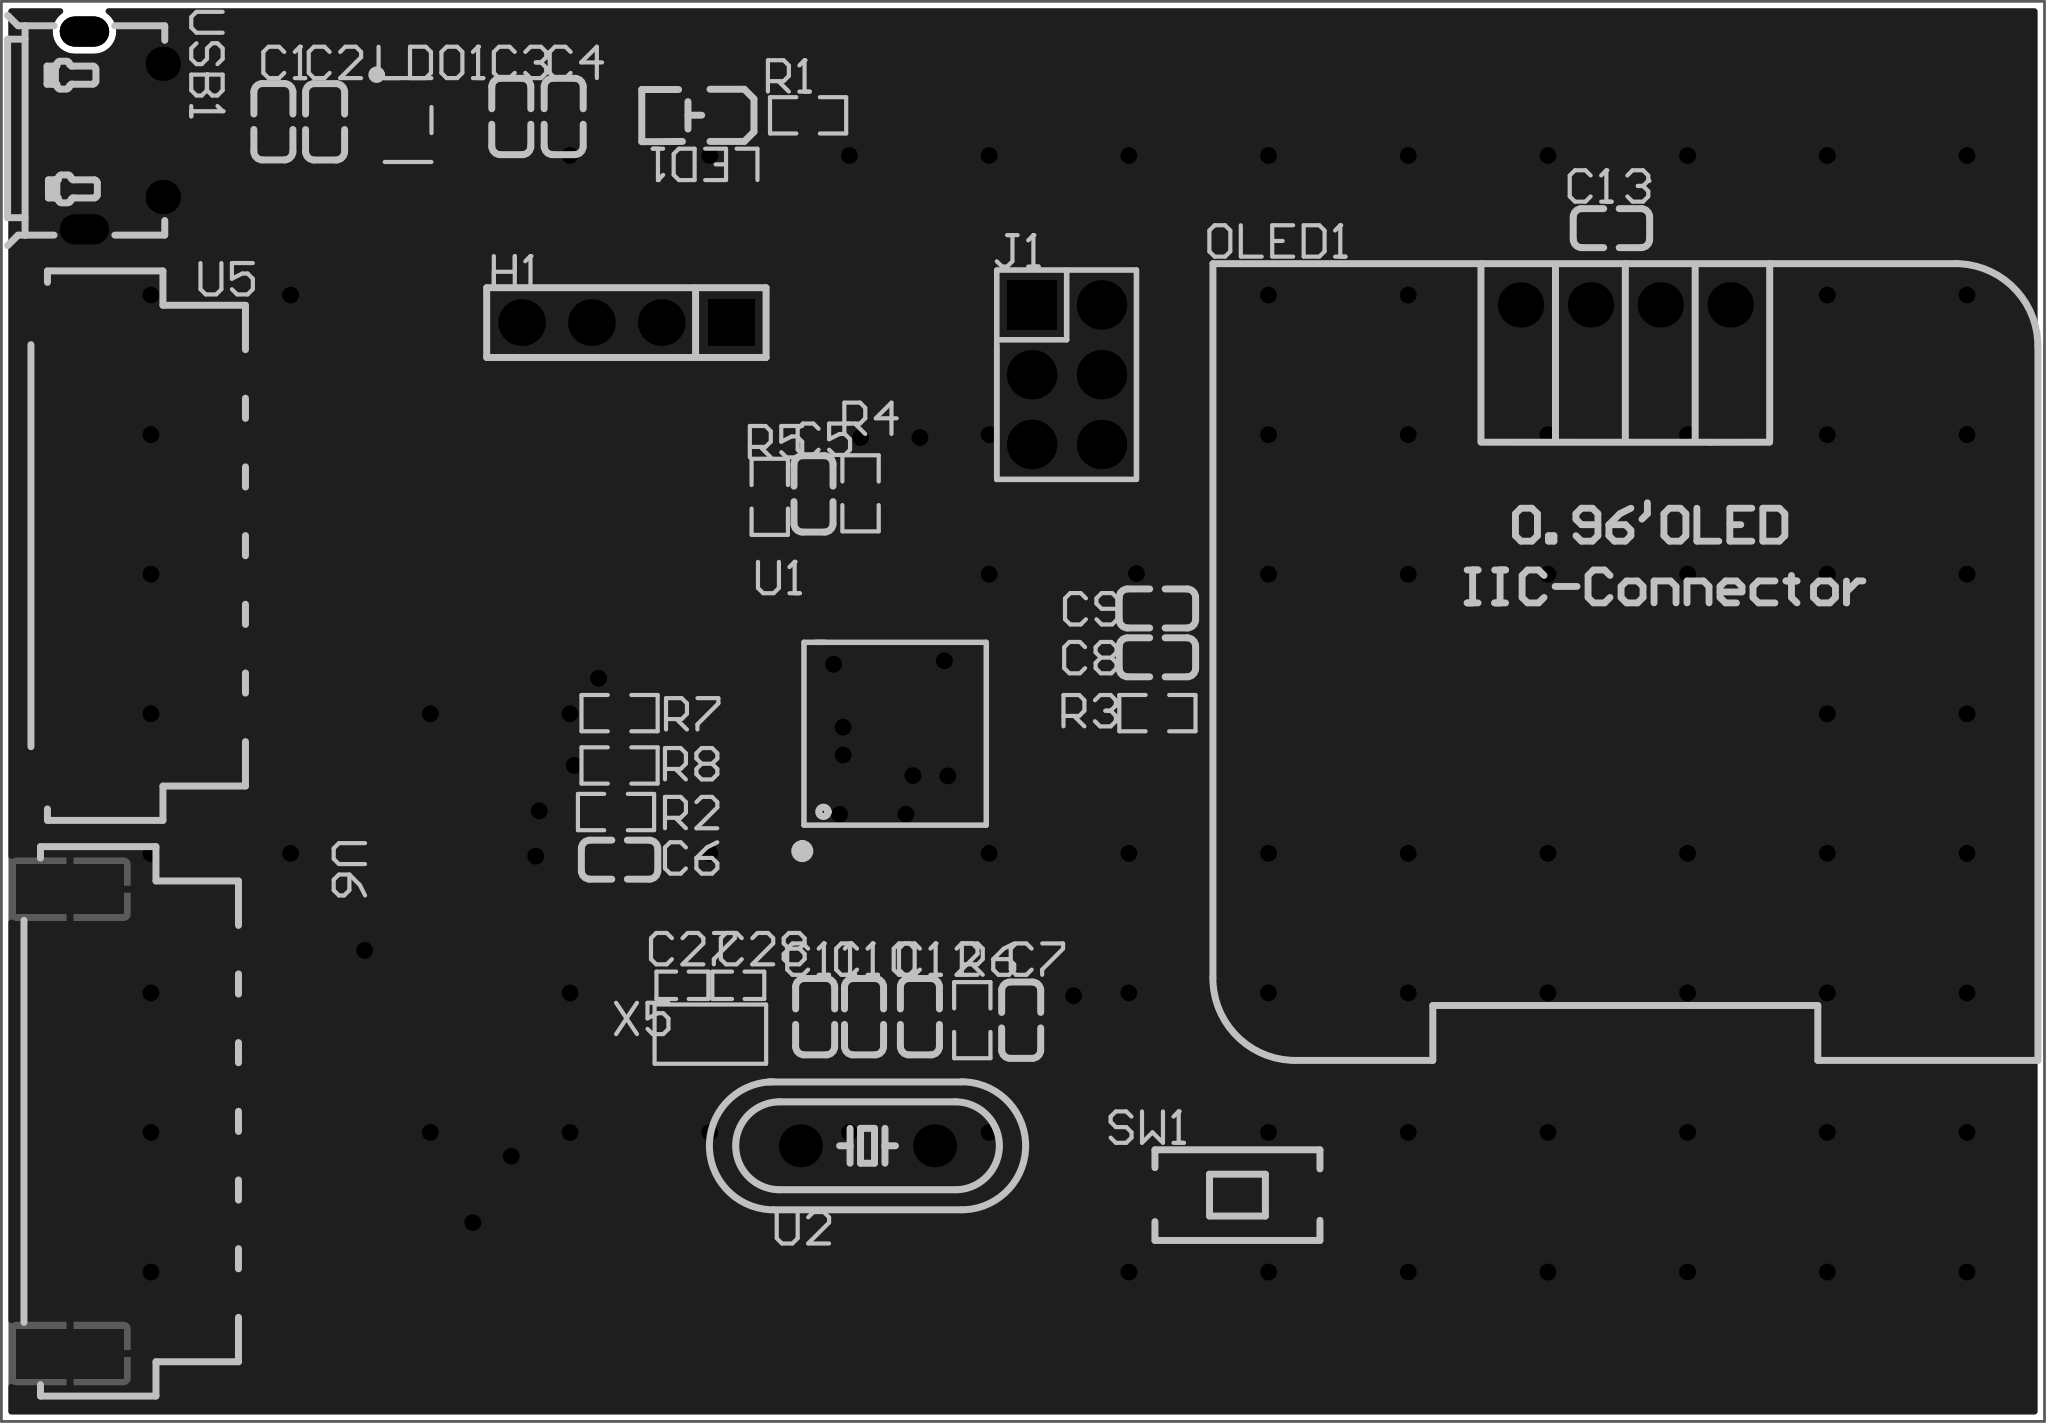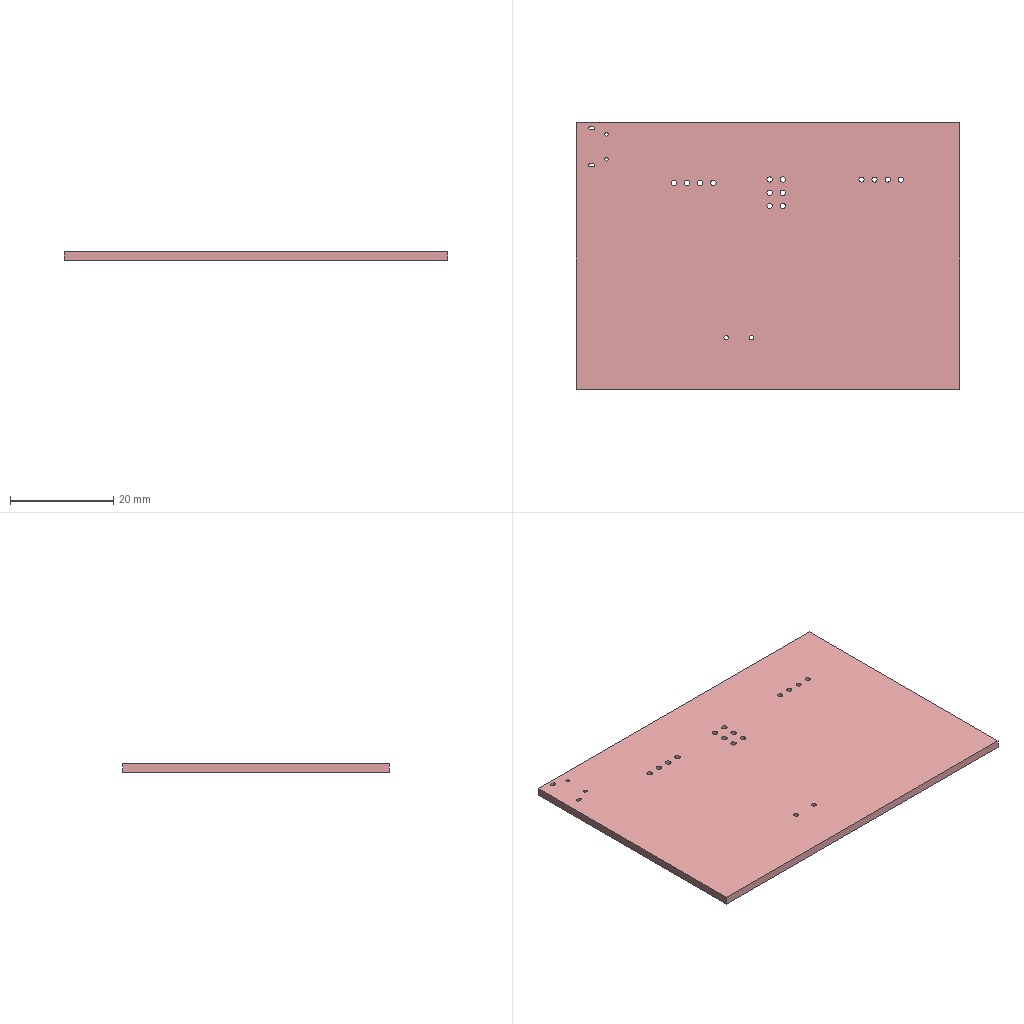Circuit board layout | Altium Designer | box 74.3 x 51.7 x 1.6 mm
Layer stack:
# Altium Designer layer stack of  (unit mm; dielectric type: 0 none, 1 core, 2 prepreg, 3 surface material)
index,name,kind,layer,copper_thickness_mm,dielectric_type,dielectric_thickness_mm,dielectric_material,dielectric_constant
0,Top Paste Mask Layer,other,,,,,,
1,Top Silkscreen Layer,other,,,,,,
2,Top Solder Mask Layer,dielectric,,,3,0.01,,3.3
3,Top Layer,copper,Top Layer,0.035,,,,
4,Dielectric1,dielectric,,,3,1.51,FR4,4.5
5,Bottom Layer,copper,Bottom Layer,0.035,,,,
6,Bottom Solder Mask Layer,dielectric,,,3,0.01,,3.3
7,Bottom Silkscreen Layer,other,,,,,,
8,Bottom Paste Mask Layer,other,,,,,,
# drill layer pairs: low layer,high layer
drill_pair,Top Layer,Bottom Layer
Part placement:
Designator,Comment,Layer,Footprint,Center-X(mm),Center-Y(mm),Rotation
C1,0.1UF,TopLayer,C0603,92.06,131.635,270
C2,1uF,TopLayer,C0603,93.94,131.632,270
C3,0.1UF,TopLayer,C0603,100.711,131.826,90
C4,1uF,TopLayer,C0603,102.616,131.826,90
C5,100nF,TopLayer,C0603,111.7,118.089,270
C6,100nF,TopLayer,C0603,104.648,104.775,0
C7,100nF,TopLayer,C0603,119.253,98.933,90
C8,100nF,TopLayer,C0603,124.206,112.141,180
C9,100nF,TopLayer,C0603,124.206,113.919,180
C10,1uF,TopLayer,C0603,113.538,99.06,270
C11,1uF,TopLayer,C0603,111.76,99.06,270
C12,0.1UF,TopLayer,C0603,115.57,99.06,90
H1,PZ254V-11-04P,TopLayer,HDR-TH_4P-P2.54-V-M,104.896,124.324,180
J1,2.54-2*3P pin header,TopLayer,HDR-TH_6P-P2.54-V-M-R2-C3-S2.54-1,120.904,122.428,270
LDO1,ME6211C33M5G-N,TopLayer,SOT-23-5_L3.0-W1.7-P0.95-LS2.8-BL,96.957,131.697,270
LED1,NCD0805R1,TopLayer,LED0805-RD,107.436,131.868,180
R1,1K,TopLayer,R0603,111.504,131.868,0
R2,10kΩ,TopLayer,R0603,104.519,106.509,180
R3,10kΩ,TopLayer,R0603,124.206,110.109,180
R4,10K,TopLayer,R0603,113.411,118.11,90
R5,10K,TopLayer,R0603,110.109,117.983,270
R6,10K,TopLayer,R0603,117.475,98.933,90
SW1,KEY_RESET,TopLayer,SW-SMD_L6.0-W3.3-LS8.0,127.254,92.583,0
U1,STM32F103C8T6,TopLayer,LQFP-48_L7.0-W7.0-P0.50-LS9.0-BL,114.681,109.347,0
U2,8M crystal,TopLayer,HC-49S_L11.5-W4.7-P4.88,113.665,94.361,0
USB1,MICRO-USB-1,TopLayer,MICRO-USB-SMD_C9900008946,86.614,131.318,270
OLED1,0.96OLED_4P_MODULE_JX,TopLayer,0.96OLED_4P,141.224,124.968,0
R7,4.7K,TopLayer,R0603,104.648,110.109,180
R8,4.7K,TopLayer,R0603,104.648,108.204,180
U5,XH2.54mm-LI-6P,TopLayer,CONN-SMD_6P-P2.50-H,88.519,116.205,270
U6,XH2.54mm-LI-6P,TopLayer,CONN-SMD_6P-P2.50-H,88.265,95.25,270
C13,0.1UF,TopLayer,C0603,140.716,127.762,0
C27,12pF,TopLayer,R0402,106.934,100.203,0
C28,12pF,TopLayer,R0402,108.966,100.203,180
X5,32.768kHz,TopLayer,OSC-SMD_L3.2-W1.5,107.95,98.425,0
Pad and via stacks:
# Altium Designer via and pad stacks of  (unit mm). Each distinct definition once, with the count of objects using it.
# via: kind,start_layer,end_layer,hole_mm,diameter_mm,mode(0 simple;1 top-mid-bottom;2 full stack),diameter_per_layer,count,example_net
# pad: kind,layer,hole_mm,hole_type(0 round;1 square;2 slot),plating,top_size,top_shape(1 round;2 rect;3 octagon;9 rounded rect),mid_size,bottom_size,mode,footprint,size_per_layer,count,example
pad,Top Layer,0,0,plated,0.8x0.9,2,0.8x0.9,0.8x0.9,0,C0603,,26,C1.2
pad,Top Layer,0,0,plated,0.49x1.157,2,0.49x1.157,0.49x1.157,0,SOT-23-5_L3.0-W1.7-P0.95-LS2.8-BL,,3,LDO1.1
pad,Top Layer,0,0,plated,0.49x1.175,2,0.49x1.175,0.49x1.175,0,SOT-23-5_L3.0-W1.7-P0.95-LS2.8-BL,,2,LDO1.4
pad,Top Layer,0,0,plated,1x1.25,2,1x1.25,1x1.25,0,LED0805-RD,,2,LED1.2
pad,Top Layer,0,0,plated,0.8065x0.864,2,0.8065x0.864,0.8065x0.864,0,R0603,,16,R1.2
pad,Top Layer,0,0,plated,1.9x1.5,2,1.9x1.5,1.9x1.5,0,SW-SMD_L6.0-W3.3-LS8.0,,2,SW1.1
pad,Top Layer,0,0,plated,0.27x1.5,1,0.27x1.5,0.27x1.5,0,LQFP-48_L7.0-W7.0-P0.50-LS9.0-BL,,24,U1.1
pad,Top Layer,0,0,plated,1.5x0.27,1,1.5x0.27,1.5x0.27,0,LQFP-48_L7.0-W7.0-P0.50-LS9.0-BL,,24,U1.13
pad,Top Layer,0,0,plated,1.35x0.4,2,1.35x0.4,1.35x0.4,0,MICRO-USB-SMD_C9900008946,,5,USB1.1
pad,Top Layer,0,0,plated,1.3x4.3,2,1.3x4.3,1.3x4.3,0,CONN-SMD_6P-P2.50-H,,12,U5.1
pad,Top Layer,0,0,plated,1.8x3.9,2,1.8x3.9,1.8x3.9,0,CONN-SMD_6P-P2.50-H,,4,U5.7
pad,Top Layer,0,0,plated,0.5657x0.54,2,0.5657x0.54,0.5657x0.54,0,R0402,,4,C27.2
pad,Top Layer,0,0,plated,1.05x1.7,2,1.05x1.7,1.05x1.7,0,OSC-SMD_L3.2-W1.5,,2,X5.1
pad,Multi-Layer,1.1,0,plated,1.7x1.7,2,1.7x1.7,1.7x1.7,0,HDR-TH_4P-P2.54-V-M,,1,H1.1
pad,Multi-Layer,1.1,0,plated,1.7x1.7,1,1.7x1.7,1.7x1.7,0,HDR-TH_4P-P2.54-V-M,,3,H1.2
pad,Multi-Layer,1.05,0,plated,1.8x1.8,1,1.8x1.8,1.8x1.8,0,HDR-TH_6P-P2.54-V-M-R2-C3-S2.54-1,,5,J1.6
pad,Multi-Layer,1.05,0,plated,1.8x1.8,2,1.8x1.8,1.8x1.8,0,HDR-TH_6P-P2.54-V-M-R2-C3-S2.54-1,,1,J1.1
pad,Multi-Layer,0.9,0,plated,1.56x1.56,1,1.56x1.56,1.56x1.56,0,HC-49S_L11.5-W4.7-P4.88,,2,U2.2
pad,Multi-Layer,0.7,0,plated,1.25x1.25,1,1.25x1.25,1.25x1.25,0,MICRO-USB-SMD_C9900008946,,2,USB1.6
pad,Multi-Layer,0.6,2,plated,1.1x1.8,1,1.1x1.8,1.1x1.8,0,MICRO-USB-SMD_C9900008946,,2,USB1.6
pad,Multi-Layer,1,0,plated,1.65x1.65,1,1.65x1.65,1.65x1.65,0,0.96OLED_4P,,4,OLED1.4
via,Top Layer,Bottom Layer,0.3048,0.61,0,,97,PB6
Copper pours:
name,layer,net,type(0 solid;1 hatched;2 none)
Top Layer-GND,Top Layer,GND,0
Bottom Layer-GND,Bottom Layer,GND,0